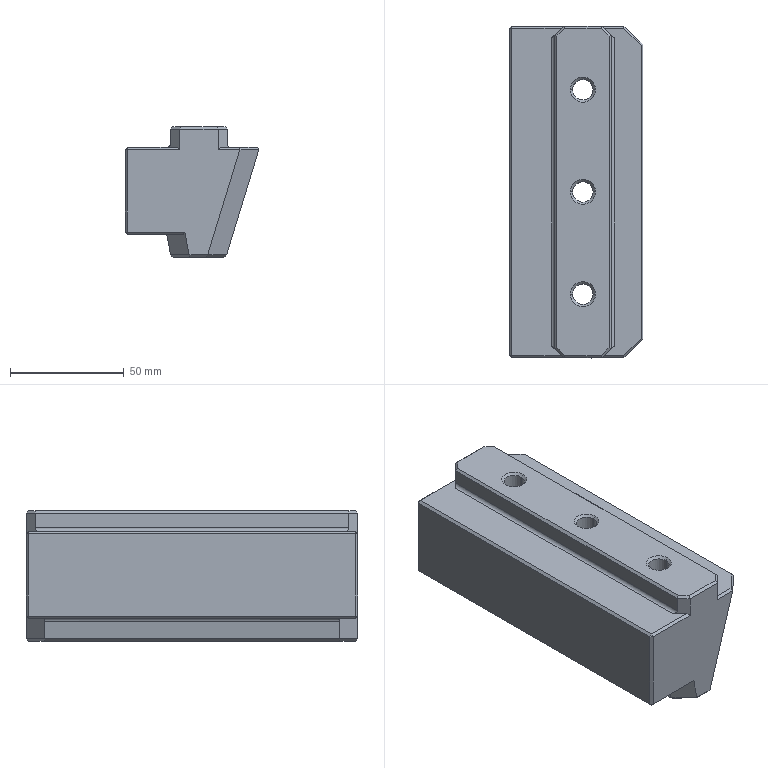Part | Creo | 1 solid | 83 faces | box 58.91 x 146 x 57.328 mm | volume 352181 mm3 | plane 56 | cylinder 15 | cone 12 | commonest cylinder face diameters 9 x6 14 x6 3 x3